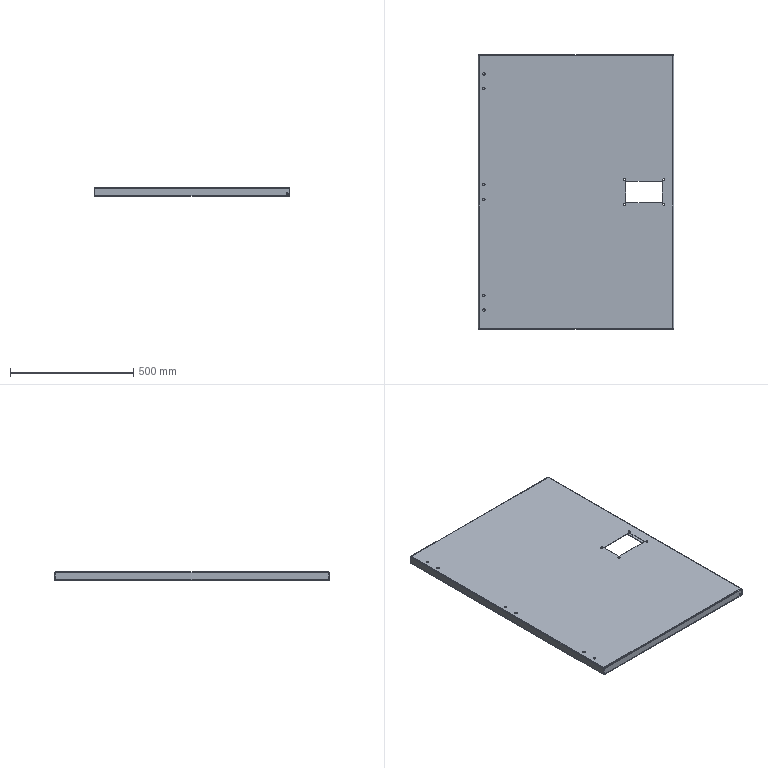Part | STEP file | SYL_0392D6J1SYL0380DJ10-1332741 | 1 solid | 130 faces | box 794 x 1114 x 35 mm | volume 2143366 mm3 | plane 78 | cylinder 44 | spline 8 | commonest cylinder face diameters 8 x12 10.5 x12 4 x8 9 x8 6 x4